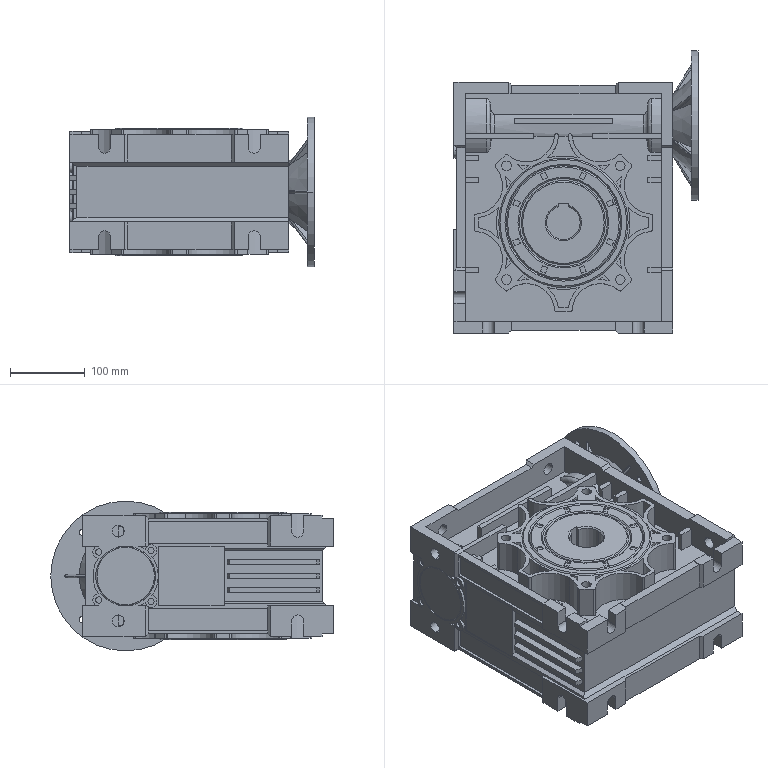Part | SolidWorks | features Boss 16, Cut 16, Fillet 5, CirPattern 3, Chamfer 2, Revolution 2, MirrorPattern 1 | 1 solid | 776 faces | box 326.25 x 377.5 x 200 mm | volume 11644494 mm3 | plane 469 | cylinder 251 | cone 28 | torus 28 | commonest cylinder face diameters 5.184 x42 85.927 x36 16 x28 178.45 x26 75.559 x20 12.8 x16